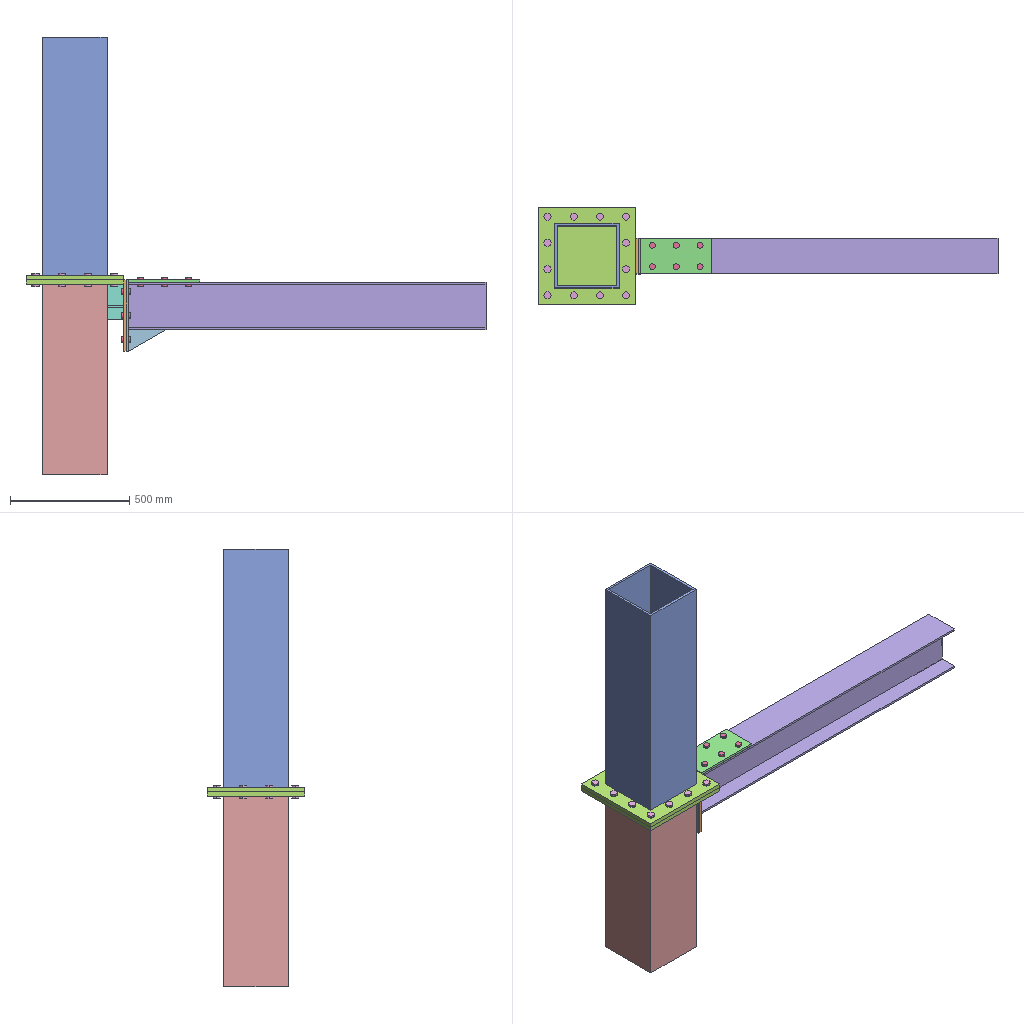Assembly | SolidWorks | 10 different items | 34 placed | box 1930 x 410 x 1836 mm
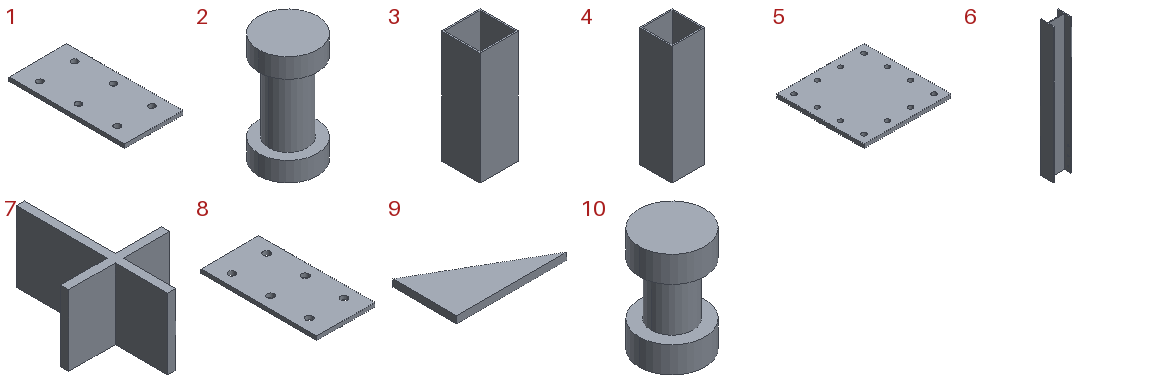Parts list (item | quantity | size | volume | features):
1 | x1 | 150 x 300 x 10 mm | 437936 mm3 | features Extrusion 1
2 | x12 | 30 x 30 x 56 mm | 25447 mm3 | features ICE 2, Extrusion 1
3 | x1 | 270 x 270 x 800 mm | 8320000 mm3 | features ExtruThin 1
4 | x1 | 270 x 270 x 1000 mm | 10400000 mm3 | features ExtruThin 1
5 | x2 | 410 x 410 x 18 mm | 2943691 mm3 | features Extrusion 1, ICE 1
6 | x1 | 200 x 150 x 1500 mm | 5674259 mm3 | features Extrusion 1, ICE 1
7 | x1 | 100 x 150 x 70 mm | 135520 mm3 | features Extrusion 1
8 | x2 | 150 x 300 x 10 mm | 434732 mm3 | features Extrusion 1
9 | x1 | 155.885 x 90 x 10 mm | 70148 mm3 | features Extrusion 1
10 | x12 | 25 x 25 x 40 mm | 13839 mm3 | features ICE 2, Extrusion 1
Mates (type | each side: item.copy, entity, surface, feature):
Coincident | 3.1 face plane Extrude-Thin1 | 5.1 face plane Boss-Extrude1
Parallel | 3.1 face plane Extrude-Thin1 | 5.1 face plane Boss-Extrude1
Width | 5.1 face plane Boss-Extrude1 | 5.1 face plane Boss-Extrude1 | 3.1 face plane Extrude-Thin1 | 3.1 face plane Extrude-Thin1 | 2 times
Coincident | 5.1 face plane Boss-Extrude1 | 5.2 face plane Boss-Extrude1 | 3 times
Coincident | 4.1 face plane Extrude-Thin1 | 5.2 face plane Boss-Extrude1
Coincident | 3.1 face plane Extrude-Thin1 | 4.1 face plane Extrude-Thin1 | 2 times
Concentric | 5.1 face cylinder Cut-Extrude1 | 2.1 face cylinder Boss-Extrude1
Coincident | 5.2 face plane Boss-Extrude1 | 2.1 face plane Boss-Extrude2
Coincident | 5.1 face plane Boss-Extrude1 | 7.1 face plane Boss-Extrude1
Coincident | 3.1 face plane Extrude-Thin1 | 7.1 face plane Boss-Extrude1
Width | 3.1 face plane Extrude-Thin1 | 3.1 face plane Extrude-Thin1 | 7.1 face plane Boss-Extrude1 | 7.1 face plane Boss-Extrude1
Coincident | 7.1 face plane Boss-Extrude1 | 8.1 face plane Boss-Extrude1
Width | 3.1 face plane Extrude-Thin1 | 3.1 face plane Extrude-Thin1 | 8.1 face plane Boss-Extrude1 | 8.1 face plane Boss-Extrude1
Coincident | 5.1 edge | 8.1 face plane Boss-Extrude1
Coincident | 8.1 face plane Boss-Extrude1 | 8.2 face plane Boss-Extrude1 | 3 times
Coincident | 8.2 face plane Boss-Extrude1 | 6.1 face plane Boss-Extrude1
Width | 3.1 face plane Extrude-Thin1 | 3.1 face plane Extrude-Thin1 | 6.1 face plane Boss-Extrude1 | 6.1 face plane Boss-Extrude1
Coincident | 6.1 face plane Boss-Extrude1 | 1.1 face plane Boss-Extrude1
Concentric | 6.1 edge | 1.1 face cylinder Boss-Extrude1
Concentric | 6.1 edge | 1.1 edge
Coincident | 8.2 face plane Boss-Extrude1 | 1.1 face plane Boss-Extrude1
Concentric | 8.2 face cylinder Boss-Extrude1 | 10.1 face cylinder Boss-Extrude1
Coincident | 8.2 face plane Boss-Extrude1 | 10.1 face plane Boss-Extrude3
Concentric | 8.2 edge | 10.2 face cylinder Boss-Extrude1
Coincident | 8.2 face plane Boss-Extrude1 | 10.2 face plane Boss-Extrude3
Coincident | 8.2 face plane Boss-Extrude1 | 9.1 face plane Boss-Extrude1
Coincident | 6.1 face plane Boss-Extrude1 | 9.1 face plane Boss-Extrude1
Width | 3.1 face plane Extrude-Thin1 | 3.1 face plane Extrude-Thin1 | 9.1 face plane Boss-Extrude1 | 9.1 face plane Boss-Extrude1
Concentric | 6.1 face cylinder Cut-Extrude1 | 10.3 face cylinder Boss-Extrude1
Width | 6.1 face plane Boss-Extrude1 | 1.1 face plane Boss-Extrude1 | 10.3 face plane Boss-Extrude3 | 10.3 face plane Boss-Extrude2
Concentric | 1.1 face cylinder Boss-Extrude1 | 10.4 face cylinder Boss-Extrude3
Coincident | 10.3 face plane Boss-Extrude3 | 10.4 face plane Boss-Extrude3